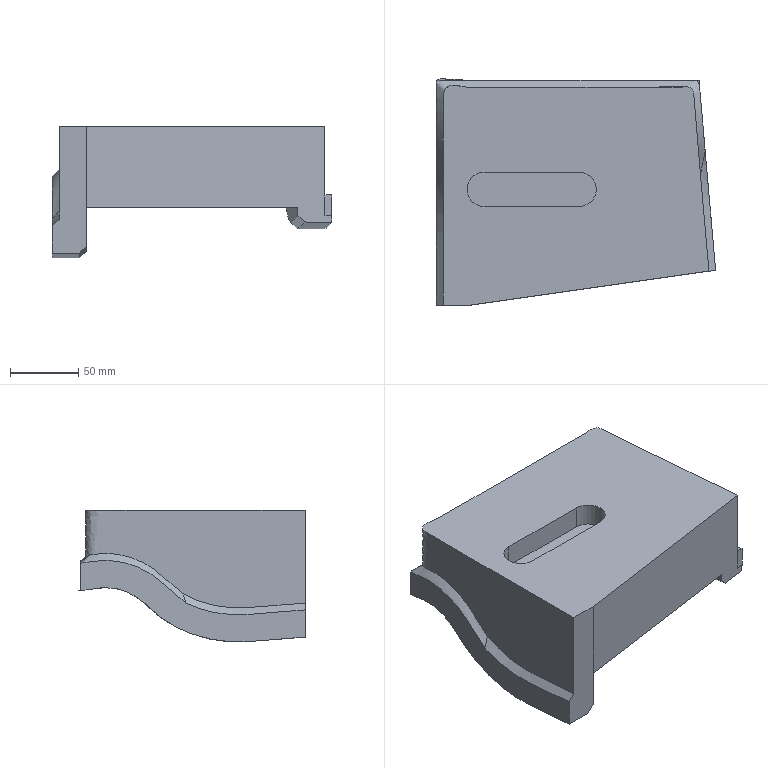Part | NX | features solid 2 | 1 solid | 47 faces | box 205.173 x 165.214 x 96.836 mm | volume 1260840 mm3 | spline 23 | plane 17 | cylinder 7 | commonest cylinder face diameters 30 x5 25 x2